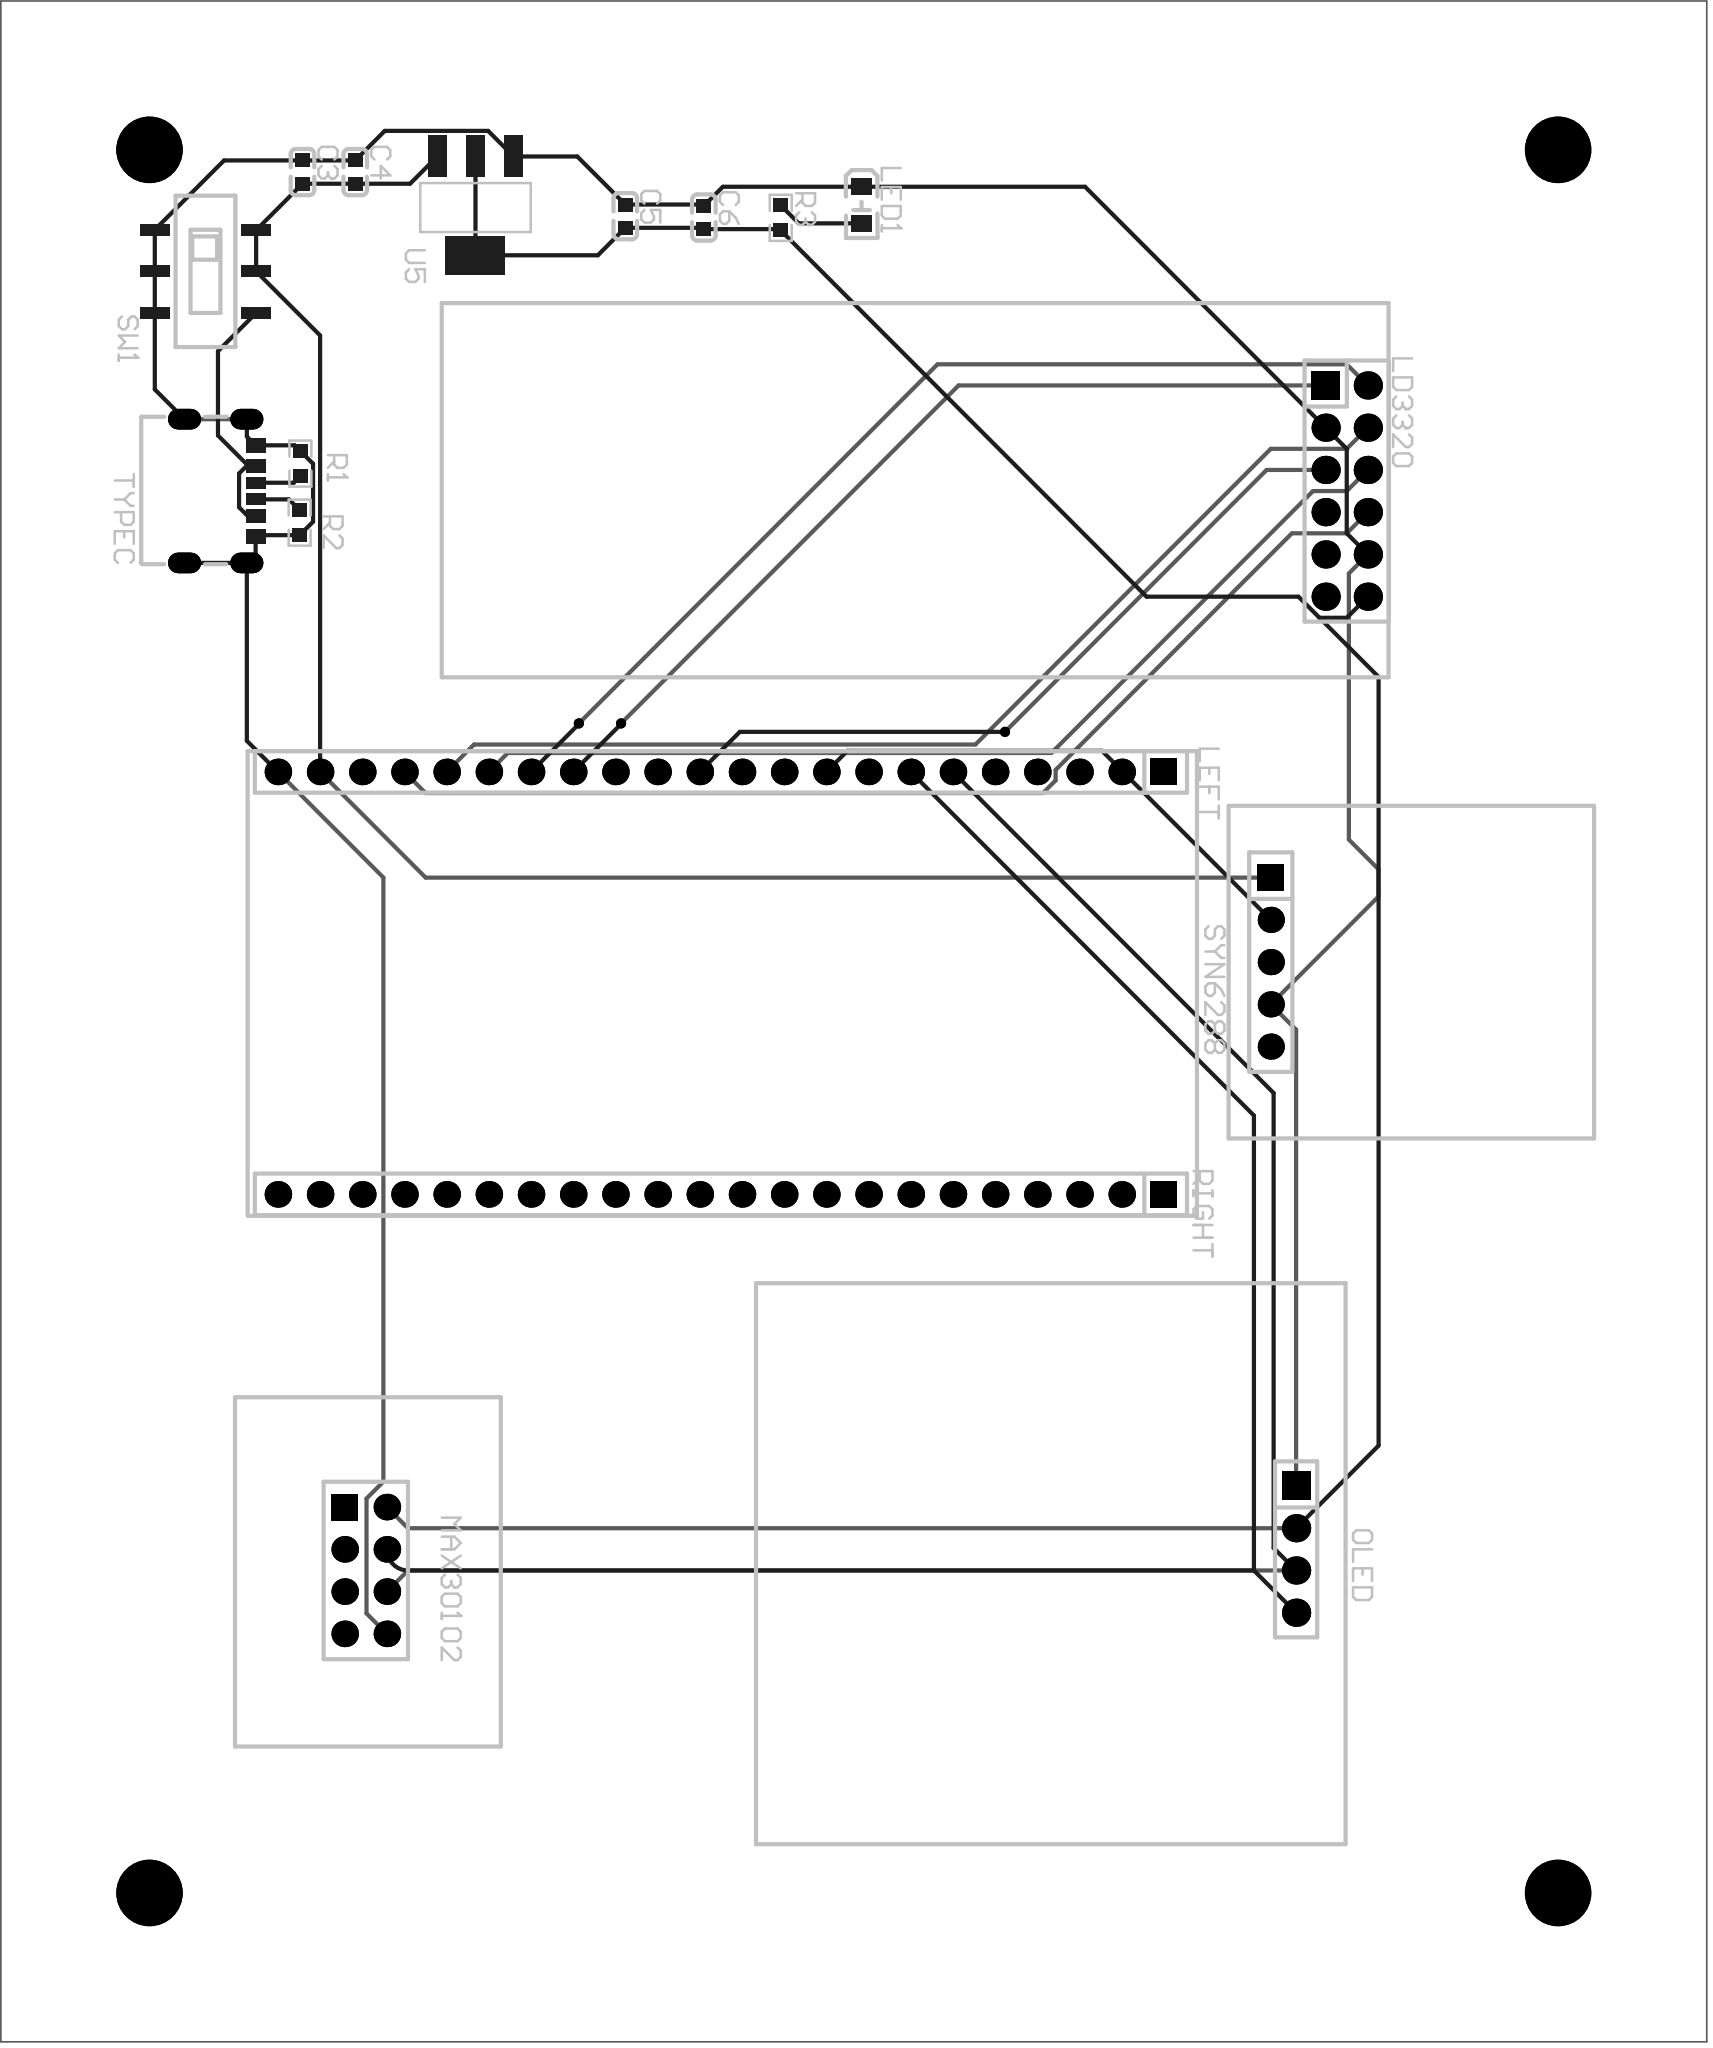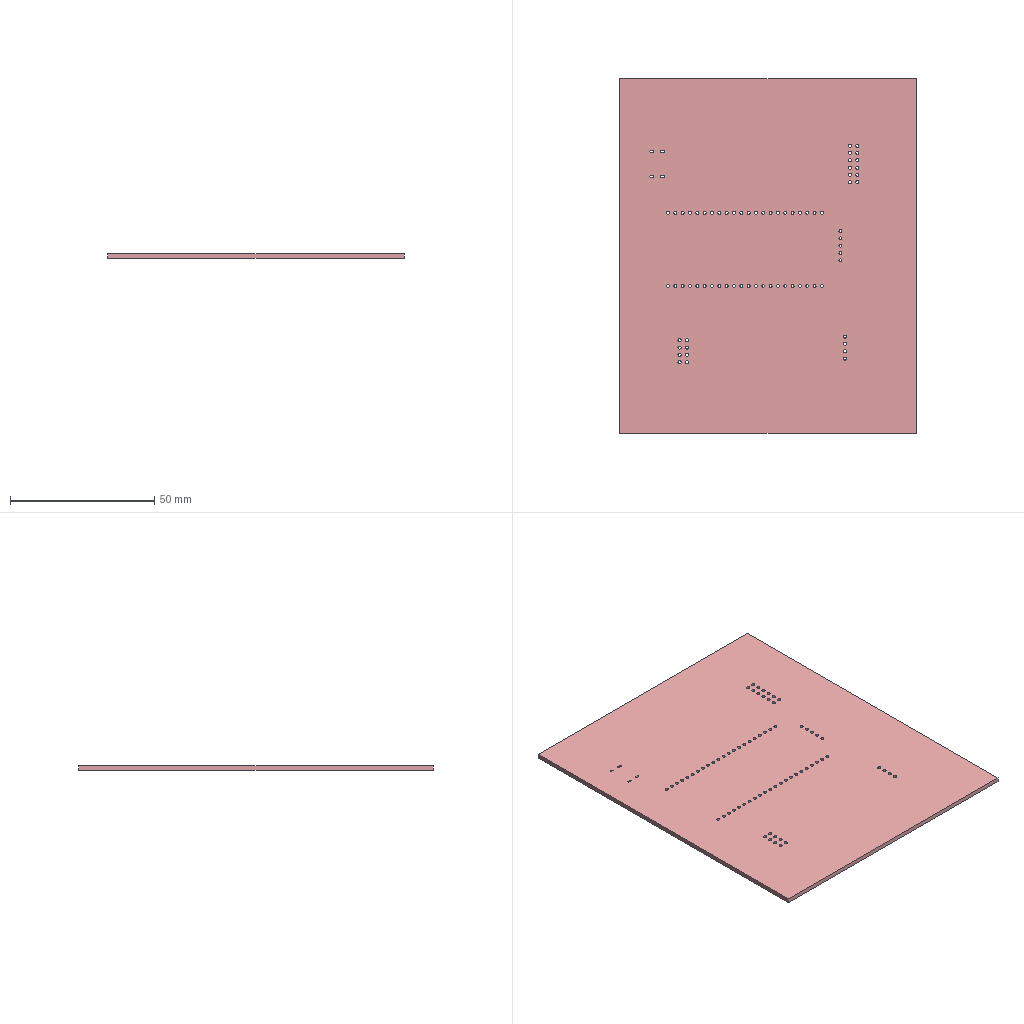Circuit board layout | Altium Designer | box 102.7 x 122.7 x 1.6 mm
Layer stack:
# Altium Designer layer stack of  (unit mm; dielectric type: 0 none, 1 core, 2 prepreg, 3 surface material)
index,name,kind,layer,copper_thickness_mm,dielectric_type,dielectric_thickness_mm,dielectric_material,dielectric_constant
0,Top Paste Mask Layer,other,,,,,,
1,Top Silkscreen Layer,other,,,,,,
2,Top Solder Mask Layer,dielectric,,,3,0.01,,3.3
3,Top Layer,copper,Top Layer,0.035,,,,
4,Dielectric1,dielectric,,,3,1.51,FR4,4.5
5,Bottom Layer,copper,Bottom Layer,0.035,,,,
6,Bottom Solder Mask Layer,dielectric,,,3,0.01,,3.3
7,Bottom Silkscreen Layer,other,,,,,,
8,Bottom Paste Mask Layer,other,,,,,,
# drill layer pairs: low layer,high layer
drill_pair,Top Layer,Bottom Layer
Part placement:
Designator,Comment,Layer,Footprint,Center-X(mm),Center-Y(mm),Rotation
C4,100nF,TopLayer,C0603,91.186,182.263,270
C6,10uf,TopLayer,C0603,112.172,179.534,270
U5,AMS1117-3.3,TopLayer,SOT-223-3_L6.5-W3.4-P2.30-LS7.0-BR,98.425,180.231,90
R1,5.1K,TopLayer,R0603,87.884,164.737,90
R2,5.1K,TopLayer,R0603,87.839,161.187,270
TYPEC,,TopLayer,USB__TYPE-C-6P,83.048,163.086,270
C3,10uF,TopLayer,C0603,88.011,182.263,270
C5,100nf,TopLayer,C0603,107.442,179.613,270
LED1,,TopLayer,LED_0805,121.671,180.281,270
R3,1K,TopLayer,R0603,116.802,179.512,90
SW1,SS-3235S-L1,TopLayer,SW-SMD_SS-3235S-LX,82.169,176.294,90
LEFT,ZX-PM2.54-1-22PY,TopLayer,HDR-TH_22P-P2.54-V-F,113.2,146.2,180
RIGHT,ZX-PM2.54-1-22PY,TopLayer,HDR-TH_22P-P2.54-V-F,113.2,120.8,180
LD3320,ZX-PM2.54-2-6PY,TopLayer,HDR-TH_12P-P2.54-V-F-R2-C6-S2.54,150.876,163.086,270
SYN6288,ZX-PM2.54-1-5PY,TopLayer,HDR-TH_5P-P2.54-V-F-B,146.304,134.765,270
MAX30102,ZX-PM2.54-2-4PY,TopLayer,HDR-TH_8P-P2.54-V-F-R2-C4-S2.54,91.821,98.189,270
OLED,ZX-PM2.54-1-4PY,TopLayer,HDR-TH_4P-P2.54-V-F,147.828,99.459,270
Pad and via stacks:
# Altium Designer via and pad stacks of  (unit mm). Each distinct definition once, with the count of objects using it.
# via: kind,start_layer,end_layer,hole_mm,diameter_mm,mode(0 simple;1 top-mid-bottom;2 full stack),diameter_per_layer,count,example_net
# pad: kind,layer,hole_mm,hole_type(0 round;1 square;2 slot),plating,top_size,top_shape(1 round;2 rect;3 octagon;9 rounded rect),mid_size,bottom_size,mode,footprint,size_per_layer,count,example
pad,Top Layer,0,0,plated,0.8x0.9,2,0.8x0.9,0.8x0.9,0,C0603,,8,C4.2
pad,Top Layer,0,0,plated,2.5x1.1,2,2.5x1.1,2.5x1.1,0,SOT-223-3_L6.5-W3.4-P2.30-LS7.0-BR,,3,U5.1
pad,Top Layer,0,0,plated,2.34x3.6,2,2.34x3.6,2.34x3.6,0,SOT-223-3_L6.5-W3.4-P2.30-LS7.0-BR,,1,U5.4
pad,Top Layer,0,0,plated,0.8065x0.864,2,0.8065x0.864,0.8065x0.864,0,R0603,,6,R1.2
pad,Top Layer,0,0,plated,0.7x1.2,2,0.7x1.2,0.7x1.2,0,USB_ TYPE-C-6P,,2,TYPEC.A5
pad,Top Layer,0,0,plated,0.8x1.2,2,0.8x1.2,0.8x1.2,0,USB_ TYPE-C-6P,,2,TYPEC.B9
pad,Top Layer,0,0,plated,0.9x1.2,2,0.9x1.2,0.9x1.2,0,USB_ TYPE-C-6P,,2,TYPEC.B12
pad,Top Layer,0,0,plated,1x1.25,2,1x1.25,1x1.25,0,LED_0805,,2,LED1.2
pad,Top Layer,0,0,plated,0.7x1.8,2,0.7x1.8,0.7x1.8,0,SW-SMD_SS-3235S-LX,,6,SW1.1
pad,Multi-Layer,0.6,2,plated,1.25x2,1,1.25x2,1.25x2,0,USB_ TYPE-C-6P,,4,TYPEC.8
pad,Multi-Layer,1.05,0,plated,1.6x1.6,2,1.6x1.6,1.6x1.6,0,HDR-TH_22P-P2.54-V-F,,2,LEFT.1
pad,Multi-Layer,1.05,0,plated,1.6x1.6,1,1.6x1.6,1.6x1.6,0,HDR-TH_22P-P2.54-V-F,,42,LEFT.2
pad,Multi-Layer,1.1,0,plated,1.7x1.7,2,1.7x1.7,1.7x1.7,0,HDR-TH_12P-P2.54-V-F-R2-C6-S2.54,,1,LD3320.1
pad,Multi-Layer,1.1,0,plated,1.7x1.7,1,1.7x1.7,1.7x1.7,0,HDR-TH_12P-P2.54-V-F-R2-C6-S2.54,,11,LD3320.2
pad,Multi-Layer,1.02,0,plated,1.575x1.575,1,1.575x1.575,1.575x1.575,0,HDR-TH_5P-P2.54-V-F-B,,4,SYN6288.5
pad,Multi-Layer,1.02,0,plated,1.575x1.575,2,1.575x1.575,1.575x1.575,0,HDR-TH_5P-P2.54-V-F-B,,1,SYN6288.1
pad,Multi-Layer,1.1,0,plated,1.6x1.6,2,1.6x1.6,1.6x1.6,0,HDR-TH_8P-P2.54-V-F-R2-C4-S2.54,,1,MAX30102.1
pad,Multi-Layer,1.1,0,plated,1.6x1.6,1,1.6x1.6,1.6x1.6,0,HDR-TH_8P-P2.54-V-F-R2-C4-S2.54,,7,MAX30102.2
pad,Multi-Layer,1.1,0,plated,1.7x1.7,2,1.7x1.7,1.7x1.7,0,HDR-TH_4P-P2.54-V-F,,1,OLED.1
pad,Multi-Layer,1.1,0,plated,1.7x1.7,1,1.7x1.7,1.7x1.7,0,HDR-TH_4P-P2.54-V-F,,3,OLED.2
via,Top Layer,Bottom Layer,3,4,0,,4,
via,Top Layer,Bottom Layer,0.3048,0.61,0,,3,IO8